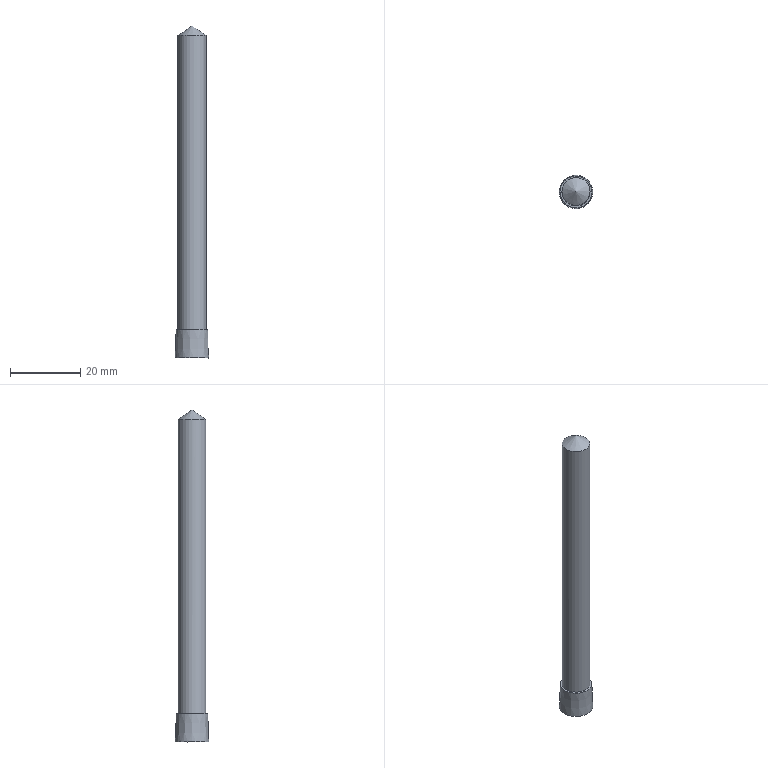Part | STEP file | 车灯-后视镜_id170_x_t | 1 solid | 5 faces | box 9.556 x 9.556 x 94.778 mm | volume 4817 mm3 | plane 2 | cone 2 | cylinder 1 | commonest cylinder face diameters 8 x1
STEP:
#1=CARTESIAN_POINT('',(-143.096,56.513,-27.286));
#2=VERTEX_POINT('',#1);
#3=CARTESIAN_POINT('',(-139.223,57.512,-27.286));
#4=DIRECTION('',(0.,0.,-1.));
#5=DIRECTION('',(-0.9683,-0.2497,0.));
#6=AXIS2_PLACEMENT_3D('',#3,#4,#5);
#7=CIRCLE('',#6,4.);
#8=EDGE_CURVE('',#2,#2,#7,.T.);
#9=ORIENTED_EDGE('',*,*,#8,.T.);
#10=EDGE_LOOP('',(#9));
#11=FACE_BOUND('',#10,.T.);
#12=CARTESIAN_POINT('',(-134.832,58.644,-27.286));
#13=VERTEX_POINT('',#12);
#14=CARTESIAN_POINT('',(-139.223,57.512,-27.286));
#15=DIRECTION('',(0.,0.,1.));
#16=DIRECTION('',(0.9683,0.2497,0.));
#17=AXIS2_PLACEMENT_3D('',#14,#15,#16);
#18=CIRCLE('',#17,4.535);
#19=EDGE_CURVE('',#13,#13,#18,.T.);
#20=ORIENTED_EDGE('',*,*,#19,.T.);
#21=EDGE_LOOP('',(#20));
#22=FACE_BOUND('',#21,.T.);
#23=CARTESIAN_POINT('',(-139.223,57.512,-27.286));
#24=DIRECTION('',(0.,0.,1.));
#25=DIRECTION('',(-0.9683,-0.2497,0.));
#26=AXIS2_PLACEMENT_3D('',#23,#24,#25);
#27=PLANE('',#26);
#28=ADVANCED_FACE('',(#11,#22),#27,.T.);
#29=CARTESIAN_POINT('',(-134.445,57.512,-35.286));
#30=VERTEX_POINT('',#29);
#31=CARTESIAN_POINT('',(-139.223,57.512,-35.286));
#32=DIRECTION('',(0.,0.,-1.));
#33=DIRECTION('',(1.,0.,0.));
#34=AXIS2_PLACEMENT_3D('',#31,#32,#33);
#35=CIRCLE('',#34,4.778);
#36=EDGE_CURVE('',#30,#30,#35,.T.);
#37=ORIENTED_EDGE('',*,*,#36,.F.);
#38=EDGE_LOOP('',(#37));
#39=FACE_BOUND('',#38,.T.);
#40=ORIENTED_EDGE('',*,*,#19,.F.);
#41=EDGE_LOOP('',(#40));
#42=FACE_BOUND('',#41,.T.);
#43=CARTESIAN_POINT('',(-139.223,57.512,-27.286));
#44=DIRECTION('',(0.,0.,-1.));
#45=DIRECTION('',(0.9683,0.2497,0.));
#46=AXIS2_PLACEMENT_3D('',#43,#44,#45);
#47=CONICAL_SURFACE('',#46,4.535,1.738);
#48=ADVANCED_FACE('',(#39,#42),#47,.T.);
#49=ORIENTED_EDGE('',*,*,#8,.F.);
#50=EDGE_LOOP('',(#49));
#51=FACE_BOUND('',#50,.T.);
#52=CARTESIAN_POINT('',(-143.223,57.512,56.794));
#53=VERTEX_POINT('',#52);
#54=CARTESIAN_POINT('',(-139.223,57.512,56.794));
#55=DIRECTION('',(0.,0.,1.));
#56=DIRECTION('',(-1.,0.,0.));
#57=AXIS2_PLACEMENT_3D('',#54,#55,#56);
#58=CIRCLE('',#57,4.);
#59=EDGE_CURVE('',#53,#53,#58,.T.);
#60=ORIENTED_EDGE('',*,*,#59,.F.);
#61=EDGE_LOOP('',(#60));
#62=FACE_BOUND('',#61,.T.);
#63=CARTESIAN_POINT('',(-139.223,57.512,-34.206));
#64=DIRECTION('',(0.,0.,1.));
#65=DIRECTION('',(-0.9683,-0.2497,0.));
#66=AXIS2_PLACEMENT_3D('',#63,#64,#65);
#67=CYLINDRICAL_SURFACE('',#66,4.);
#68=ADVANCED_FACE('',(#51,#62),#67,.T.);
#69=ORIENTED_EDGE('',*,*,#59,.T.);
#70=EDGE_LOOP('',(#69));
#71=FACE_BOUND('',#70,.T.);
#72=CARTESIAN_POINT('',(-139.223,57.512,59.492));
#73=VERTEX_POINT('',#72);
#74=VERTEX_LOOP('',#73);
#75=FACE_BOUND('',#74,.T.);
#76=CARTESIAN_POINT('',(-139.223,57.512,59.492));
#77=DIRECTION('',(0.,0.,-1.));
#78=DIRECTION('',(-0.9683,-0.2497,0.));
#79=AXIS2_PLACEMENT_3D('',#76,#77,#78);
#80=CONICAL_SURFACE('',#79,0.,56.);
#81=ADVANCED_FACE('',(#71,#75),#80,.T.);
#82=ORIENTED_EDGE('',*,*,#36,.T.);
#83=EDGE_LOOP('',(#82));
#84=FACE_OUTER_BOUND('',#83,.T.);
#85=CARTESIAN_POINT('',(-139.223,57.512,-35.286));
#86=DIRECTION('',(0.,0.,1.));
#87=DIRECTION('',(0.9683,0.2497,0.));
#88=AXIS2_PLACEMENT_3D('',#85,#86,#87);
#89=PLANE('',#88);
#90=ADVANCED_FACE('',(#84),#89,.F.);
#91=CLOSED_SHELL('',(#28,#48,#68,#81,#90));
#92=MANIFOLD_SOLID_BREP('',#91);
#93=(LENGTH_UNIT()NAMED_UNIT(*)SI_UNIT(.MILLI.,.METRE.));
#94=UNCERTAINTY_MEASURE_WITH_UNIT(LENGTH_MEASURE(0.00002),#93,'','');
#95=(NAMED_UNIT(*)PLANE_ANGLE_UNIT()SI_UNIT($,.RADIAN.));
#96=PLANE_ANGLE_MEASURE_WITH_UNIT(PLANE_ANGLE_MEASURE(0.01745),#95);
#97=DIMENSIONAL_EXPONENTS(0.,0.,0.,0.,0.,0.,0.);
#98=(CONVERSION_BASED_UNIT('DEGREE',#96)NAMED_UNIT(#97)PLANE_ANGLE_UNIT());
#99=(NAMED_UNIT(*)SI_UNIT($,.STERADIAN.)SOLID_ANGLE_UNIT());
#100=(GEOMETRIC_REPRESENTATION_CONTEXT(3)GLOBAL_UNCERTAINTY_ASSIGNED_CONTEXT((#94))GLOBAL_UNIT_ASSIGNED_CONTEXT((#93,#98,#99))REPRESENTATION_CONTEXT('',''));
#101=ADVANCED_BREP_SHAPE_REPRESENTATION('',(#92),#100);